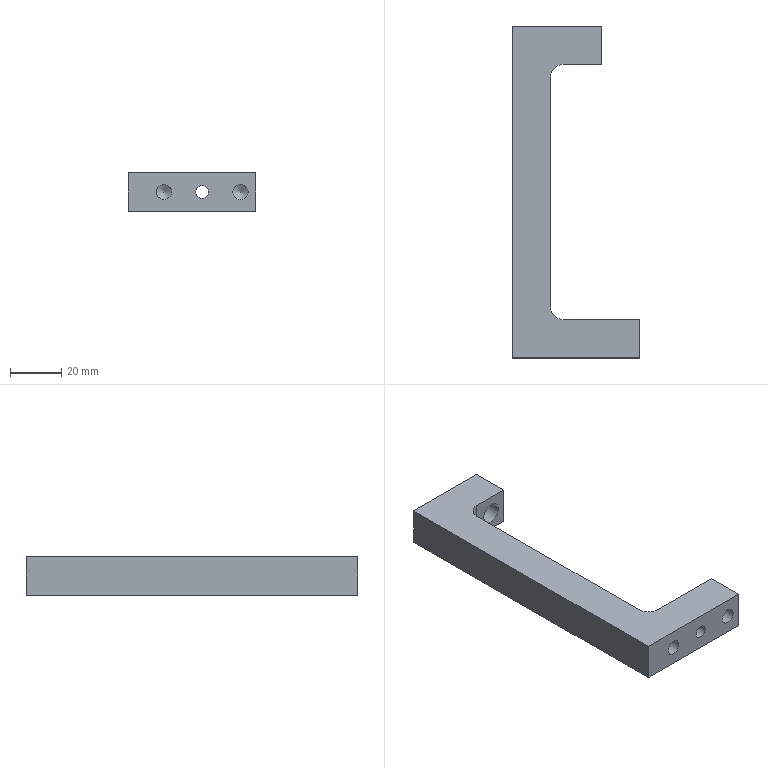Part | NX | features BREP 1 | 1 solid | 18 faces | box 50 x 130 x 15 mm | volume 40025 mm3 | plane 10 | cylinder 6 | cone 2 | commonest cylinder face diameters 6 x2 10 x2 5 x1 8 x1
STEP:
#1=CARTESIAN_POINT('',(50.,15.,15.));
#2=VERTEX_POINT('',#1);
#3=CARTESIAN_POINT('',(50.,0.,15.));
#4=VERTEX_POINT('',#3);
#5=CARTESIAN_POINT('',(50.,0.,15.));
#6=DIRECTION('',(0.,-1.,0.));
#7=VECTOR('',#6,1000.);
#8=LINE('',#5,#7);
#9=EDGE_CURVE('',#2,#4,#8,.T.);
#10=ORIENTED_EDGE('',*,*,#9,.F.);
#11=CARTESIAN_POINT('',(20.,15.,15.));
#12=VERTEX_POINT('',#11);
#13=CARTESIAN_POINT('',(0.,15.,15.));
#14=DIRECTION('',(1.,0.,0.));
#15=VECTOR('',#14,1000.);
#16=LINE('',#13,#15);
#17=EDGE_CURVE('',#12,#2,#16,.T.);
#18=ORIENTED_EDGE('',*,*,#17,.F.);
#19=CARTESIAN_POINT('',(15.,20.,15.));
#20=VERTEX_POINT('',#19);
#21=CARTESIAN_POINT('',(20.,20.,15.));
#22=DIRECTION('',(0.,0.,1.));
#23=DIRECTION('',(1.,0.,0.));
#24=AXIS2_PLACEMENT_3D('',#21,#22,#23);
#25=CIRCLE('',#24,5.);
#26=EDGE_CURVE('',#20,#12,#25,.T.);
#27=ORIENTED_EDGE('',*,*,#26,.F.);
#28=CARTESIAN_POINT('',(15.,110.,15.));
#29=VERTEX_POINT('',#28);
#30=CARTESIAN_POINT('',(15.,0.,15.));
#31=DIRECTION('',(0.,-1.,0.));
#32=VECTOR('',#31,1000.);
#33=LINE('',#30,#32);
#34=EDGE_CURVE('',#29,#20,#33,.T.);
#35=ORIENTED_EDGE('',*,*,#34,.F.);
#36=CARTESIAN_POINT('',(20.,115.,15.));
#37=VERTEX_POINT('',#36);
#38=CARTESIAN_POINT('',(20.,110.,15.));
#39=DIRECTION('',(0.,0.,1.));
#40=DIRECTION('',(1.,0.,0.));
#41=AXIS2_PLACEMENT_3D('',#38,#39,#40);
#42=CIRCLE('',#41,5.);
#43=EDGE_CURVE('',#37,#29,#42,.T.);
#44=ORIENTED_EDGE('',*,*,#43,.F.);
#45=CARTESIAN_POINT('',(35.,115.,15.));
#46=VERTEX_POINT('',#45);
#47=CARTESIAN_POINT('',(0.,115.,15.));
#48=DIRECTION('',(-1.,0.,0.));
#49=VECTOR('',#48,1000.);
#50=LINE('',#47,#49);
#51=EDGE_CURVE('',#46,#37,#50,.T.);
#52=ORIENTED_EDGE('',*,*,#51,.F.);
#53=CARTESIAN_POINT('',(35.,130.,15.));
#54=VERTEX_POINT('',#53);
#55=CARTESIAN_POINT('',(35.,0.,15.));
#56=DIRECTION('',(0.,-1.,0.));
#57=VECTOR('',#56,1000.);
#58=LINE('',#55,#57);
#59=EDGE_CURVE('',#54,#46,#58,.T.);
#60=ORIENTED_EDGE('',*,*,#59,.F.);
#61=CARTESIAN_POINT('',(0.,130.,15.));
#62=VERTEX_POINT('',#61);
#63=CARTESIAN_POINT('',(0.,130.,15.));
#64=DIRECTION('',(1.,0.,0.));
#65=VECTOR('',#64,1000.);
#66=LINE('',#63,#65);
#67=EDGE_CURVE('',#62,#54,#66,.T.);
#68=ORIENTED_EDGE('',*,*,#67,.F.);
#69=CARTESIAN_POINT('',(0.,0.,15.));
#70=VERTEX_POINT('',#69);
#71=CARTESIAN_POINT('',(0.,0.,15.));
#72=DIRECTION('',(0.,1.,0.));
#73=VECTOR('',#72,1000.);
#74=LINE('',#71,#73);
#75=EDGE_CURVE('',#70,#62,#74,.T.);
#76=ORIENTED_EDGE('',*,*,#75,.F.);
#77=CARTESIAN_POINT('',(0.,0.,15.));
#78=DIRECTION('',(-1.,0.,0.));
#79=VECTOR('',#78,1000.);
#80=LINE('',#77,#79);
#81=EDGE_CURVE('',#4,#70,#80,.T.);
#82=ORIENTED_EDGE('',*,*,#81,.F.);
#83=EDGE_LOOP('',(#10,#18,#27,#35,#44,#52,#60,#68,#76,#82));
#84=FACE_BOUND('',#83,.T.);
#85=CARTESIAN_POINT('',(0.,0.,15.));
#86=DIRECTION('',(0.,0.,-1.));
#87=DIRECTION('',(1.,0.,0.));
#88=AXIS2_PLACEMENT_3D('',#85,#86,#87);
#89=PLANE('',#88);
#90=ADVANCED_FACE('',(#84),#89,.F.);
#91=CARTESIAN_POINT('',(50.,0.,0.));
#92=VERTEX_POINT('',#91);
#93=CARTESIAN_POINT('',(50.,0.,15.));
#94=DIRECTION('',(0.,0.,-1.));
#95=VECTOR('',#94,1000.);
#96=LINE('',#93,#95);
#97=EDGE_CURVE('',#4,#92,#96,.T.);
#98=ORIENTED_EDGE('',*,*,#97,.F.);
#99=ORIENTED_EDGE('',*,*,#81,.T.);
#100=CARTESIAN_POINT('',(0.,0.,0.));
#101=VERTEX_POINT('',#100);
#102=CARTESIAN_POINT('',(0.,0.,15.));
#103=DIRECTION('',(0.,0.,1.));
#104=VECTOR('',#103,1000.);
#105=LINE('',#102,#104);
#106=EDGE_CURVE('',#101,#70,#105,.T.);
#107=ORIENTED_EDGE('',*,*,#106,.F.);
#108=CARTESIAN_POINT('',(50.,0.,0.));
#109=DIRECTION('',(-1.,0.,0.));
#110=VECTOR('',#109,1000.);
#111=LINE('',#108,#110);
#112=EDGE_CURVE('',#92,#101,#111,.T.);
#113=ORIENTED_EDGE('',*,*,#112,.F.);
#114=EDGE_LOOP('',(#98,#99,#107,#113));
#115=FACE_BOUND('',#114,.T.);
#116=CARTESIAN_POINT('',(14.,0.,4.5));
#117=VERTEX_POINT('',#116);
#118=CARTESIAN_POINT('',(14.,0.,7.5));
#119=DIRECTION('',(0.,-1.,0.));
#120=DIRECTION('',(0.,0.,-1.));
#121=AXIS2_PLACEMENT_3D('',#118,#119,#120);
#122=CIRCLE('',#121,3.);
#123=EDGE_CURVE('',#117,#117,#122,.T.);
#124=ORIENTED_EDGE('',*,*,#123,.F.);
#125=EDGE_LOOP('',(#124));
#126=FACE_BOUND('',#125,.T.);
#127=CARTESIAN_POINT('',(44.,0.,4.5));
#128=VERTEX_POINT('',#127);
#129=CARTESIAN_POINT('',(44.,0.,7.5));
#130=DIRECTION('',(0.,-1.,0.));
#131=DIRECTION('',(0.,0.,-1.));
#132=AXIS2_PLACEMENT_3D('',#129,#130,#131);
#133=CIRCLE('',#132,3.);
#134=EDGE_CURVE('',#128,#128,#133,.T.);
#135=ORIENTED_EDGE('',*,*,#134,.F.);
#136=EDGE_LOOP('',(#135));
#137=FACE_BOUND('',#136,.T.);
#138=CARTESIAN_POINT('',(29.,0.,5.));
#139=VERTEX_POINT('',#138);
#140=CARTESIAN_POINT('',(29.,0.,7.5));
#141=DIRECTION('',(0.,-1.,0.));
#142=DIRECTION('',(0.,0.,-1.));
#143=AXIS2_PLACEMENT_3D('',#140,#141,#142);
#144=CIRCLE('',#143,2.5);
#145=EDGE_CURVE('',#139,#139,#144,.T.);
#146=ORIENTED_EDGE('',*,*,#145,.F.);
#147=EDGE_LOOP('',(#146));
#148=FACE_BOUND('',#147,.T.);
#149=CARTESIAN_POINT('',(50.,0.,15.));
#150=DIRECTION('',(0.,1.,0.));
#151=DIRECTION('',(1.,0.,0.));
#152=AXIS2_PLACEMENT_3D('',#149,#150,#151);
#153=PLANE('',#152);
#154=ADVANCED_FACE('',(#115,#126,#137,#148),#153,.F.);
#155=CARTESIAN_POINT('',(50.,15.,0.));
#156=VERTEX_POINT('',#155);
#157=CARTESIAN_POINT('',(50.,15.,15.));
#158=DIRECTION('',(0.,0.,-1.));
#159=VECTOR('',#158,1000.);
#160=LINE('',#157,#159);
#161=EDGE_CURVE('',#2,#156,#160,.T.);
#162=ORIENTED_EDGE('',*,*,#161,.F.);
#163=ORIENTED_EDGE('',*,*,#9,.T.);
#164=ORIENTED_EDGE('',*,*,#97,.T.);
#165=CARTESIAN_POINT('',(50.,15.,0.));
#166=DIRECTION('',(0.,-1.,0.));
#167=VECTOR('',#166,1000.);
#168=LINE('',#165,#167);
#169=EDGE_CURVE('',#156,#92,#168,.T.);
#170=ORIENTED_EDGE('',*,*,#169,.F.);
#171=EDGE_LOOP('',(#162,#163,#164,#170));
#172=FACE_BOUND('',#171,.T.);
#173=CARTESIAN_POINT('',(50.,15.,15.));
#174=DIRECTION('',(-1.,0.,0.));
#175=DIRECTION('',(0.,0.,-1.));
#176=AXIS2_PLACEMENT_3D('',#173,#174,#175);
#177=PLANE('',#176);
#178=ADVANCED_FACE('',(#172),#177,.F.);
#179=CARTESIAN_POINT('',(20.,15.,0.));
#180=VERTEX_POINT('',#179);
#181=CARTESIAN_POINT('',(20.,15.,15.));
#182=DIRECTION('',(0.,0.,-1.));
#183=VECTOR('',#182,1000.);
#184=LINE('',#181,#183);
#185=EDGE_CURVE('',#12,#180,#184,.T.);
#186=ORIENTED_EDGE('',*,*,#185,.F.);
#187=ORIENTED_EDGE('',*,*,#17,.T.);
#188=ORIENTED_EDGE('',*,*,#161,.T.);
#189=CARTESIAN_POINT('',(15.,15.,0.));
#190=DIRECTION('',(1.,0.,0.));
#191=VECTOR('',#190,1000.);
#192=LINE('',#189,#191);
#193=EDGE_CURVE('',#180,#156,#192,.T.);
#194=ORIENTED_EDGE('',*,*,#193,.F.);
#195=EDGE_LOOP('',(#186,#187,#188,#194));
#196=FACE_BOUND('',#195,.T.);
#197=CARTESIAN_POINT('',(29.,15.,5.));
#198=VERTEX_POINT('',#197);
#199=CARTESIAN_POINT('',(29.,15.,7.5));
#200=DIRECTION('',(0.,1.,0.));
#201=DIRECTION('',(0.,0.,-1.));
#202=AXIS2_PLACEMENT_3D('',#199,#200,#201);
#203=CIRCLE('',#202,2.5);
#204=EDGE_CURVE('',#198,#198,#203,.T.);
#205=ORIENTED_EDGE('',*,*,#204,.F.);
#206=EDGE_LOOP('',(#205));
#207=FACE_BOUND('',#206,.T.);
#208=CARTESIAN_POINT('',(15.,15.,15.));
#209=DIRECTION('',(0.,-1.,0.));
#210=DIRECTION('',(0.,0.,1.));
#211=AXIS2_PLACEMENT_3D('',#208,#209,#210);
#212=PLANE('',#211);
#213=ADVANCED_FACE('',(#196,#207),#212,.F.);
#214=ORIENTED_EDGE('',*,*,#185,.T.);
#215=CARTESIAN_POINT('',(15.,20.,0.));
#216=VERTEX_POINT('',#215);
#217=CARTESIAN_POINT('',(20.,20.,0.));
#218=DIRECTION('',(0.,0.,1.));
#219=DIRECTION('',(1.,0.,0.));
#220=AXIS2_PLACEMENT_3D('',#217,#218,#219);
#221=CIRCLE('',#220,5.);
#222=EDGE_CURVE('',#216,#180,#221,.T.);
#223=ORIENTED_EDGE('',*,*,#222,.F.);
#224=CARTESIAN_POINT('',(15.,20.,15.));
#225=DIRECTION('',(0.,0.,-1.));
#226=VECTOR('',#225,1000.);
#227=LINE('',#224,#226);
#228=EDGE_CURVE('',#20,#216,#227,.T.);
#229=ORIENTED_EDGE('',*,*,#228,.F.);
#230=ORIENTED_EDGE('',*,*,#26,.T.);
#231=EDGE_LOOP('',(#214,#223,#229,#230));
#232=FACE_BOUND('',#231,.T.);
#233=CARTESIAN_POINT('',(20.,20.,15.));
#234=DIRECTION('',(0.,0.,1.));
#235=DIRECTION('',(-1.,0.,0.));
#236=AXIS2_PLACEMENT_3D('',#233,#234,#235);
#237=CYLINDRICAL_SURFACE('',#236,5.);
#238=ADVANCED_FACE('',(#232),#237,.F.);
#239=CARTESIAN_POINT('',(15.,110.,0.));
#240=VERTEX_POINT('',#239);
#241=CARTESIAN_POINT('',(15.,110.,15.));
#242=DIRECTION('',(0.,0.,-1.));
#243=VECTOR('',#242,1000.);
#244=LINE('',#241,#243);
#245=EDGE_CURVE('',#29,#240,#244,.T.);
#246=ORIENTED_EDGE('',*,*,#245,.F.);
#247=ORIENTED_EDGE('',*,*,#34,.T.);
#248=ORIENTED_EDGE('',*,*,#228,.T.);
#249=CARTESIAN_POINT('',(15.,115.,0.));
#250=DIRECTION('',(0.,-1.,0.));
#251=VECTOR('',#250,1000.);
#252=LINE('',#249,#251);
#253=EDGE_CURVE('',#240,#216,#252,.T.);
#254=ORIENTED_EDGE('',*,*,#253,.F.);
#255=EDGE_LOOP('',(#246,#247,#248,#254));
#256=FACE_BOUND('',#255,.T.);
#257=CARTESIAN_POINT('',(15.,115.,15.));
#258=DIRECTION('',(-1.,0.,0.));
#259=DIRECTION('',(0.,1.,0.));
#260=AXIS2_PLACEMENT_3D('',#257,#258,#259);
#261=PLANE('',#260);
#262=ADVANCED_FACE('',(#256),#261,.F.);
#263=ORIENTED_EDGE('',*,*,#245,.T.);
#264=CARTESIAN_POINT('',(20.,115.,0.));
#265=VERTEX_POINT('',#264);
#266=CARTESIAN_POINT('',(20.,110.,0.));
#267=DIRECTION('',(0.,0.,1.));
#268=DIRECTION('',(1.,0.,0.));
#269=AXIS2_PLACEMENT_3D('',#266,#267,#268);
#270=CIRCLE('',#269,5.);
#271=EDGE_CURVE('',#265,#240,#270,.T.);
#272=ORIENTED_EDGE('',*,*,#271,.F.);
#273=CARTESIAN_POINT('',(20.,115.,15.));
#274=DIRECTION('',(0.,0.,-1.));
#275=VECTOR('',#274,1000.);
#276=LINE('',#273,#275);
#277=EDGE_CURVE('',#37,#265,#276,.T.);
#278=ORIENTED_EDGE('',*,*,#277,.F.);
#279=ORIENTED_EDGE('',*,*,#43,.T.);
#280=EDGE_LOOP('',(#263,#272,#278,#279));
#281=FACE_BOUND('',#280,.T.);
#282=CARTESIAN_POINT('',(20.,110.,15.));
#283=DIRECTION('',(0.,0.,1.));
#284=DIRECTION('',(-1.,0.,0.));
#285=AXIS2_PLACEMENT_3D('',#282,#283,#284);
#286=CYLINDRICAL_SURFACE('',#285,5.);
#287=ADVANCED_FACE('',(#281),#286,.F.);
#288=ORIENTED_EDGE('',*,*,#277,.T.);
#289=CARTESIAN_POINT('',(35.,115.,0.));
#290=VERTEX_POINT('',#289);
#291=CARTESIAN_POINT('',(35.,115.,0.));
#292=DIRECTION('',(-1.,0.,0.));
#293=VECTOR('',#292,1000.);
#294=LINE('',#291,#293);
#295=EDGE_CURVE('',#290,#265,#294,.T.);
#296=ORIENTED_EDGE('',*,*,#295,.F.);
#297=CARTESIAN_POINT('',(35.,115.,15.));
#298=DIRECTION('',(0.,0.,-1.));
#299=VECTOR('',#298,1000.);
#300=LINE('',#297,#299);
#301=EDGE_CURVE('',#46,#290,#300,.T.);
#302=ORIENTED_EDGE('',*,*,#301,.F.);
#303=ORIENTED_EDGE('',*,*,#51,.T.);
#304=EDGE_LOOP('',(#288,#296,#302,#303));
#305=FACE_BOUND('',#304,.T.);
#306=CARTESIAN_POINT('',(28.,115.,11.5));
#307=VERTEX_POINT('',#306);
#308=CARTESIAN_POINT('',(28.,115.,7.5));
#309=DIRECTION('',(0.,-1.,0.));
#310=DIRECTION('',(0.,0.,1.));
#311=AXIS2_PLACEMENT_3D('',#308,#309,#310);
#312=CIRCLE('',#311,4.);
#313=EDGE_CURVE('',#307,#307,#312,.T.);
#314=ORIENTED_EDGE('',*,*,#313,.F.);
#315=EDGE_LOOP('',(#314));
#316=FACE_BOUND('',#315,.T.);
#317=CARTESIAN_POINT('',(35.,115.,15.));
#318=DIRECTION('',(0.,1.,0.));
#319=DIRECTION('',(0.,0.,-1.));
#320=AXIS2_PLACEMENT_3D('',#317,#318,#319);
#321=PLANE('',#320);
#322=ADVANCED_FACE('',(#305,#316),#321,.F.);
#323=CARTESIAN_POINT('',(35.,130.,0.));
#324=VERTEX_POINT('',#323);
#325=CARTESIAN_POINT('',(35.,130.,15.));
#326=DIRECTION('',(0.,0.,-1.));
#327=VECTOR('',#326,1000.);
#328=LINE('',#325,#327);
#329=EDGE_CURVE('',#54,#324,#328,.T.);
#330=ORIENTED_EDGE('',*,*,#329,.F.);
#331=ORIENTED_EDGE('',*,*,#59,.T.);
#332=ORIENTED_EDGE('',*,*,#301,.T.);
#333=CARTESIAN_POINT('',(35.,130.,0.));
#334=DIRECTION('',(0.,-1.,0.));
#335=VECTOR('',#334,1000.);
#336=LINE('',#333,#335);
#337=EDGE_CURVE('',#324,#290,#336,.T.);
#338=ORIENTED_EDGE('',*,*,#337,.F.);
#339=EDGE_LOOP('',(#330,#331,#332,#338));
#340=FACE_BOUND('',#339,.T.);
#341=CARTESIAN_POINT('',(35.,130.,15.));
#342=DIRECTION('',(-1.,0.,0.));
#343=DIRECTION('',(0.,1.,0.));
#344=AXIS2_PLACEMENT_3D('',#341,#342,#343);
#345=PLANE('',#344);
#346=ADVANCED_FACE('',(#340),#345,.F.);
#347=CARTESIAN_POINT('',(28.,130.,11.5));
#348=VERTEX_POINT('',#347);
#349=CARTESIAN_POINT('',(28.,130.,7.5));
#350=DIRECTION('',(0.,1.,0.));
#351=DIRECTION('',(0.,0.,1.));
#352=AXIS2_PLACEMENT_3D('',#349,#350,#351);
#353=CIRCLE('',#352,4.);
#354=EDGE_CURVE('',#348,#348,#353,.T.);
#355=ORIENTED_EDGE('',*,*,#354,.F.);
#356=EDGE_LOOP('',(#355));
#357=FACE_BOUND('',#356,.T.);
#358=CARTESIAN_POINT('',(0.,130.,0.));
#359=VERTEX_POINT('',#358);
#360=CARTESIAN_POINT('',(0.,130.,15.));
#361=DIRECTION('',(0.,0.,-1.));
#362=VECTOR('',#361,1000.);
#363=LINE('',#360,#362);
#364=EDGE_CURVE('',#62,#359,#363,.T.);
#365=ORIENTED_EDGE('',*,*,#364,.F.);
#366=ORIENTED_EDGE('',*,*,#67,.T.);
#367=ORIENTED_EDGE('',*,*,#329,.T.);
#368=CARTESIAN_POINT('',(0.,130.,0.));
#369=DIRECTION('',(1.,0.,0.));
#370=VECTOR('',#369,1000.);
#371=LINE('',#368,#370);
#372=EDGE_CURVE('',#359,#324,#371,.T.);
#373=ORIENTED_EDGE('',*,*,#372,.F.);
#374=EDGE_LOOP('',(#365,#366,#367,#373));
#375=FACE_BOUND('',#374,.T.);
#376=CARTESIAN_POINT('',(0.,130.,15.));
#377=DIRECTION('',(0.,-1.,0.));
#378=DIRECTION('',(0.,0.,1.));
#379=AXIS2_PLACEMENT_3D('',#376,#377,#378);
#380=PLANE('',#379);
#381=ADVANCED_FACE('',(#357,#375),#380,.F.);
#382=ORIENTED_EDGE('',*,*,#106,.T.);
#383=ORIENTED_EDGE('',*,*,#75,.T.);
#384=ORIENTED_EDGE('',*,*,#364,.T.);
#385=CARTESIAN_POINT('',(0.,0.,0.));
#386=DIRECTION('',(0.,1.,0.));
#387=VECTOR('',#386,1000.);
#388=LINE('',#385,#387);
#389=EDGE_CURVE('',#101,#359,#388,.T.);
#390=ORIENTED_EDGE('',*,*,#389,.F.);
#391=EDGE_LOOP('',(#382,#383,#384,#390));
#392=FACE_BOUND('',#391,.T.);
#393=CARTESIAN_POINT('',(0.,0.,15.));
#394=DIRECTION('',(1.,0.,0.));
#395=DIRECTION('',(0.,0.,1.));
#396=AXIS2_PLACEMENT_3D('',#393,#394,#395);
#397=PLANE('',#396);
#398=ADVANCED_FACE('',(#392),#397,.F.);
#399=ORIENTED_EDGE('',*,*,#193,.T.);
#400=ORIENTED_EDGE('',*,*,#169,.T.);
#401=ORIENTED_EDGE('',*,*,#112,.T.);
#402=ORIENTED_EDGE('',*,*,#389,.T.);
#403=ORIENTED_EDGE('',*,*,#372,.T.);
#404=ORIENTED_EDGE('',*,*,#337,.T.);
#405=ORIENTED_EDGE('',*,*,#295,.T.);
#406=ORIENTED_EDGE('',*,*,#271,.T.);
#407=ORIENTED_EDGE('',*,*,#253,.T.);
#408=ORIENTED_EDGE('',*,*,#222,.T.);
#409=EDGE_LOOP('',(#399,#400,#401,#402,#403,#404,#405,#406,#407,#408));
#410=FACE_BOUND('',#409,.T.);
#411=CARTESIAN_POINT('',(0.,0.,0.));
#412=DIRECTION('',(0.,0.,-1.));
#413=DIRECTION('',(1.,0.,0.));
#414=AXIS2_PLACEMENT_3D('',#411,#412,#413);
#415=PLANE('',#414);
#416=ADVANCED_FACE('',(#410),#415,.T.);
#417=CARTESIAN_POINT('',(14.,12.,4.5));
#418=VERTEX_POINT('',#417);
#419=CARTESIAN_POINT('',(14.,12.,7.5));
#420=DIRECTION('',(0.,-1.,0.));
#421=DIRECTION('',(0.,0.,-1.));
#422=AXIS2_PLACEMENT_3D('',#419,#420,#421);
#423=CIRCLE('',#422,3.);
#424=EDGE_CURVE('',#418,#418,#423,.T.);
#425=ORIENTED_EDGE('',*,*,#424,.F.);
#426=EDGE_LOOP('',(#425));
#427=FACE_BOUND('',#426,.T.);
#428=ORIENTED_EDGE('',*,*,#123,.T.);
#429=EDGE_LOOP('',(#428));
#430=FACE_BOUND('',#429,.T.);
#431=CARTESIAN_POINT('',(14.,0.,7.5));
#432=DIRECTION('',(0.,-1.,0.));
#433=DIRECTION('',(0.,0.,1.));
#434=AXIS2_PLACEMENT_3D('',#431,#432,#433);
#435=CYLINDRICAL_SURFACE('',#434,3.);
#436=ADVANCED_FACE('',(#427,#430),#435,.F.);
#437=CARTESIAN_POINT('',(44.,12.,4.5));
#438=VERTEX_POINT('',#437);
#439=CARTESIAN_POINT('',(44.,12.,7.5));
#440=DIRECTION('',(0.,-1.,0.));
#441=DIRECTION('',(0.,0.,-1.));
#442=AXIS2_PLACEMENT_3D('',#439,#440,#441);
#443=CIRCLE('',#442,3.);
#444=EDGE_CURVE('',#438,#438,#443,.T.);
#445=ORIENTED_EDGE('',*,*,#444,.F.);
#446=EDGE_LOOP('',(#445));
#447=FACE_BOUND('',#446,.T.);
#448=ORIENTED_EDGE('',*,*,#134,.T.);
#449=EDGE_LOOP('',(#448));
#450=FACE_BOUND('',#449,.T.);
#451=CARTESIAN_POINT('',(44.,0.,7.5));
#452=DIRECTION('',(0.,-1.,0.));
#453=DIRECTION('',(0.,0.,1.));
#454=AXIS2_PLACEMENT_3D('',#451,#452,#453);
#455=CYLINDRICAL_SURFACE('',#454,3.);
#456=ADVANCED_FACE('',(#447,#450),#455,.F.);
#457=ORIENTED_EDGE('',*,*,#204,.T.);
#458=EDGE_LOOP('',(#457));
#459=FACE_BOUND('',#458,.T.);
#460=ORIENTED_EDGE('',*,*,#145,.T.);
#461=EDGE_LOOP('',(#460));
#462=FACE_BOUND('',#461,.T.);
#463=CARTESIAN_POINT('',(29.,0.,7.5));
#464=DIRECTION('',(0.,-1.,0.));
#465=DIRECTION('',(0.,0.,1.));
#466=AXIS2_PLACEMENT_3D('',#463,#464,#465);
#467=CYLINDRICAL_SURFACE('',#466,2.5);
#468=ADVANCED_FACE('',(#459,#462),#467,.F.);
#469=ORIENTED_EDGE('',*,*,#313,.T.);
#470=EDGE_LOOP('',(#469));
#471=FACE_BOUND('',#470,.T.);
#472=ORIENTED_EDGE('',*,*,#354,.T.);
#473=EDGE_LOOP('',(#472));
#474=FACE_BOUND('',#473,.T.);
#475=CARTESIAN_POINT('',(28.,130.,7.5));
#476=DIRECTION('',(0.,1.,0.));
#477=DIRECTION('',(0.,0.,-1.));
#478=AXIS2_PLACEMENT_3D('',#475,#476,#477);
#479=CYLINDRICAL_SURFACE('',#478,4.);
#480=ADVANCED_FACE('',(#471,#474),#479,.F.);
#481=CARTESIAN_POINT('',(14.,13.803,7.5));
#482=VERTEX_POINT('',#481);
#483=VERTEX_LOOP('',#482);
#484=FACE_BOUND('',#483,.T.);
#485=ORIENTED_EDGE('',*,*,#424,.T.);
#486=EDGE_LOOP('',(#485));
#487=FACE_BOUND('',#486,.T.);
#488=CARTESIAN_POINT('',(14.,12.,7.5));
#489=DIRECTION('',(0.,-1.,0.));
#490=DIRECTION('',(-1.,0.,0.));
#491=AXIS2_PLACEMENT_3D('',#488,#489,#490);
#492=CONICAL_SURFACE('',#491,3.,1.03);
#493=ADVANCED_FACE('',(#484,#487),#492,.F.);
#494=CARTESIAN_POINT('',(44.,13.803,7.5));
#495=VERTEX_POINT('',#494);
#496=VERTEX_LOOP('',#495);
#497=FACE_BOUND('',#496,.T.);
#498=ORIENTED_EDGE('',*,*,#444,.T.);
#499=EDGE_LOOP('',(#498));
#500=FACE_BOUND('',#499,.T.);
#501=CARTESIAN_POINT('',(44.,12.,7.5));
#502=DIRECTION('',(0.,-1.,0.));
#503=DIRECTION('',(0.,0.,1.));
#504=AXIS2_PLACEMENT_3D('',#501,#502,#503);
#505=CONICAL_SURFACE('',#504,3.,1.03);
#506=ADVANCED_FACE('',(#497,#500),#505,.F.);
#507=CLOSED_SHELL('',(#90,#154,#178,#213,#238,#262,#287,#322,#346,#381,#398,#416,#436,#456,#468,#480,#493,#506));
#508=MANIFOLD_SOLID_BREP('',#507);
#509=(LENGTH_UNIT()NAMED_UNIT(*)SI_UNIT(.MILLI.,.METRE.));
#510=UNCERTAINTY_MEASURE_WITH_UNIT(LENGTH_MEASURE(0.00001),#509,'','');
#511=(NAMED_UNIT(*)PLANE_ANGLE_UNIT()SI_UNIT($,.RADIAN.));
#512=(NAMED_UNIT(*)SI_UNIT($,.STERADIAN.)SOLID_ANGLE_UNIT());
#513=(GEOMETRIC_REPRESENTATION_CONTEXT(3)GLOBAL_UNCERTAINTY_ASSIGNED_CONTEXT((#510))GLOBAL_UNIT_ASSIGNED_CONTEXT((#509,#511,#512))REPRESENTATION_CONTEXT('',''));
#514=ADVANCED_BREP_SHAPE_REPRESENTATION('',(#508),#513);